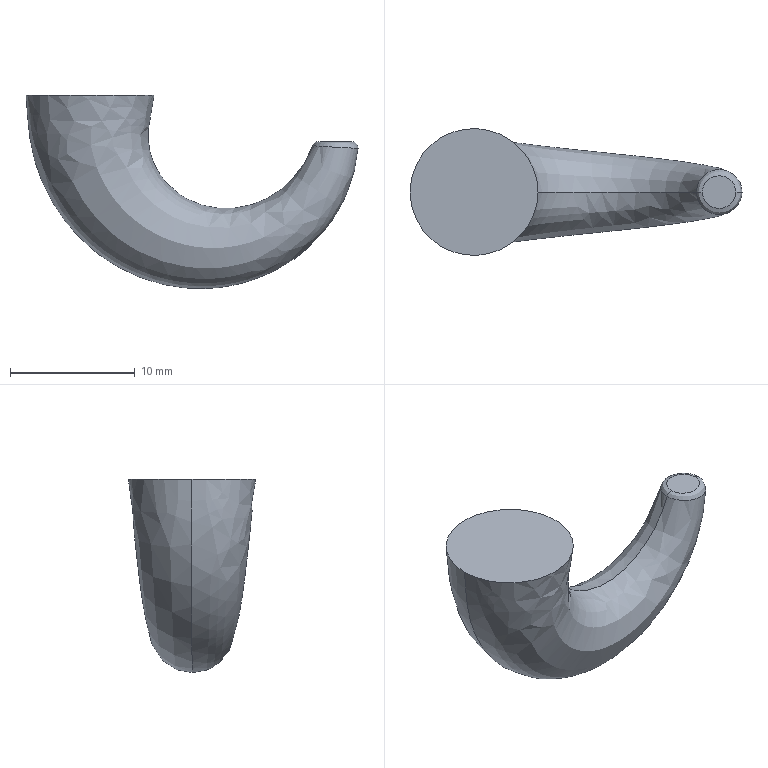Part | STEP file | solid 215 | 1 solid | 6 faces | box 26.632 x 10.173 x 15.494 mm | volume 1276 mm3 | spline 4 | plane 2